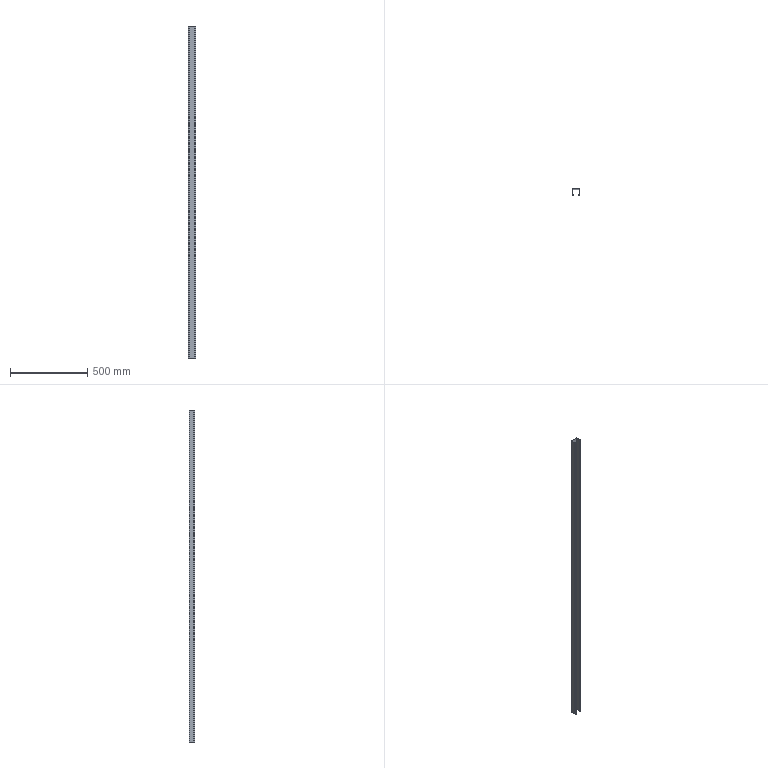Part | STEP file | 31E-01027QY25 | 1 solid | 28 faces | box 50 x 38.192 x 2150 mm | volume 353976 mm3 | plane 16 | cylinder 12 | commonest cylinder face diameters 1 x4 2 x4 4 x2 26 x2
STEP:
#1=CARTESIAN_POINT('',(27.993,8.298,1075.));
#2=VERTEX_POINT('',#1);
#3=CARTESIAN_POINT('',(32.281,3.187,1075.));
#4=VERTEX_POINT('',#3);
#5=CARTESIAN_POINT('',(30.137,5.743,1075.));
#6=DIRECTION('',(0.6428,-0.766,0.));
#7=VECTOR('',#6,1.);
#8=LINE('',#5,#7);
#9=EDGE_CURVE('',#2,#4,#8,.T.);
#10=ORIENTED_EDGE('',*,*,#9,.F.);
#11=CARTESIAN_POINT('',(27.993,8.298,-1075.));
#12=VERTEX_POINT('',#11);
#13=CARTESIAN_POINT('',(27.993,8.298,0.));
#14=DIRECTION('',(0.,0.,-1.));
#15=VECTOR('',#14,1.);
#16=LINE('',#13,#15);
#17=EDGE_CURVE('',#2,#12,#16,.T.);
#18=ORIENTED_EDGE('',*,*,#17,.T.);
#19=CARTESIAN_POINT('',(32.281,3.187,-1075.));
#20=VERTEX_POINT('',#19);
#21=CARTESIAN_POINT('',(30.137,5.743,-1075.));
#22=DIRECTION('',(0.6428,-0.766,0.));
#23=VECTOR('',#22,1.);
#24=LINE('',#21,#23);
#25=EDGE_CURVE('',#12,#20,#24,.T.);
#26=ORIENTED_EDGE('',*,*,#25,.T.);
#27=CARTESIAN_POINT('',(32.281,3.187,0.));
#28=DIRECTION('',(0.,0.,-1.));
#29=VECTOR('',#28,1.);
#30=LINE('',#27,#29);
#31=EDGE_CURVE('',#4,#20,#30,.T.);
#32=ORIENTED_EDGE('',*,*,#31,.F.);
#33=EDGE_LOOP('',(#10,#18,#26,#32));
#34=FACE_OUTER_BOUND('',#33,.T.);
#35=CARTESIAN_POINT('',(27.525,8.856,1075.));
#36=DIRECTION('',(0.766,0.6428,0.));
#37=DIRECTION('',(-0.6428,0.766,0.));
#38=AXIS2_PLACEMENT_3D('',#35,#36,#37);
#39=PLANE('',#38);
#40=ADVANCED_FACE('',(#34),#39,.F.);
#41=CARTESIAN_POINT('',(76.525,38.856,1075.));
#42=VERTEX_POINT('',#41);
#43=CARTESIAN_POINT('',(28.525,38.856,1075.));
#44=VERTEX_POINT('',#43);
#45=CARTESIAN_POINT('',(52.525,38.856,1075.));
#46=DIRECTION('',(-1.,0.,0.));
#47=VECTOR('',#46,1.);
#48=LINE('',#45,#47);
#49=EDGE_CURVE('',#42,#44,#48,.T.);
#50=ORIENTED_EDGE('',*,*,#49,.T.);
#51=CARTESIAN_POINT('',(27.525,37.856,1075.));
#52=VERTEX_POINT('',#51);
#53=CARTESIAN_POINT('',(28.525,37.856,1075.));
#54=DIRECTION('',(0.,0.,1.));
#55=AXIS2_PLACEMENT_3D('',#53,#54,$);
#56=CIRCLE('',#55,1.);
#57=EDGE_CURVE('',#44,#52,#56,.T.);
#58=ORIENTED_EDGE('',*,*,#57,.T.);
#59=CARTESIAN_POINT('',(27.525,9.584,1075.));
#60=VERTEX_POINT('',#59);
#61=CARTESIAN_POINT('',(27.525,23.72,1075.));
#62=DIRECTION('',(0.,-1.,0.));
#63=VECTOR('',#62,1.);
#64=LINE('',#61,#63);
#65=EDGE_CURVE('',#52,#60,#64,.T.);
#66=ORIENTED_EDGE('',*,*,#65,.T.);
#67=CARTESIAN_POINT('',(29.525,9.584,1075.));
#68=DIRECTION('',(0.,0.,1.));
#69=AXIS2_PLACEMENT_3D('',#67,#68,$);
#70=CIRCLE('',#69,2.);
#71=EDGE_CURVE('',#60,#2,#70,.T.);
#72=ORIENTED_EDGE('',*,*,#71,.T.);
#73=ORIENTED_EDGE('',*,*,#9,.T.);
#74=CARTESIAN_POINT('',(28.342,2.493,1075.));
#75=VERTEX_POINT('',#74);
#76=CARTESIAN_POINT('',(30.312,2.84,1075.));
#77=DIRECTION('',(-0.9848,-0.1736,0.));
#78=VECTOR('',#77,1.);
#79=LINE('',#76,#78);
#80=EDGE_CURVE('',#4,#75,#79,.T.);
#81=ORIENTED_EDGE('',*,*,#80,.T.);
#82=CARTESIAN_POINT('',(32.653,0.6877,1075.));
#83=VERTEX_POINT('',#82);
#84=CARTESIAN_POINT('',(35.437,13.386,1075.));
#85=DIRECTION('',(0.,0.,1.));
#86=AXIS2_PLACEMENT_3D('',#84,#85,$);
#87=CIRCLE('',#86,13.);
#88=EDGE_CURVE('',#75,#83,#87,.T.);
#89=ORIENTED_EDGE('',*,*,#88,.T.);
#90=CARTESIAN_POINT('',(33.867,1.665,1075.));
#91=VERTEX_POINT('',#90);
#92=CARTESIAN_POINT('',(32.867,1.665,1075.));
#93=DIRECTION('',(0.,0.,1.));
#94=AXIS2_PLACEMENT_3D('',#92,#93,$);
#95=CIRCLE('',#94,1.);
#96=EDGE_CURVE('',#83,#91,#95,.T.);
#97=ORIENTED_EDGE('',*,*,#96,.T.);
#98=CARTESIAN_POINT('',(33.867,2.983,1075.));
#99=VERTEX_POINT('',#98);
#100=CARTESIAN_POINT('',(33.867,2.324,1075.));
#101=DIRECTION('',(0.,1.,0.));
#102=VECTOR('',#101,1.);
#103=LINE('',#100,#102);
#104=EDGE_CURVE('',#91,#99,#103,.T.);
#105=ORIENTED_EDGE('',*,*,#104,.T.);
#106=CARTESIAN_POINT('',(33.75,3.304,1075.));
#107=VERTEX_POINT('',#106);
#108=CARTESIAN_POINT('',(33.367,2.983,1075.));
#109=DIRECTION('',(0.,0.,1.));
#110=AXIS2_PLACEMENT_3D('',#108,#109,$);
#111=CIRCLE('',#110,0.5);
#112=EDGE_CURVE('',#99,#107,#111,.T.);
#113=ORIENTED_EDGE('',*,*,#112,.T.);
#114=CARTESIAN_POINT('',(28.725,9.293,1075.));
#115=VERTEX_POINT('',#114);
#116=CARTESIAN_POINT('',(31.237,6.298,1075.));
#117=DIRECTION('',(-0.6428,0.766,0.));
#118=VECTOR('',#117,1.);
#119=LINE('',#116,#118);
#120=EDGE_CURVE('',#107,#115,#119,.T.);
#121=ORIENTED_EDGE('',*,*,#120,.T.);
#122=CARTESIAN_POINT('',(28.725,37.156,1075.));
#123=VERTEX_POINT('',#122);
#124=CARTESIAN_POINT('',(28.725,23.225,1075.));
#125=DIRECTION('',(0.,1.,0.));
#126=VECTOR('',#125,1.);
#127=LINE('',#124,#126);
#128=EDGE_CURVE('',#115,#123,#127,.T.);
#129=ORIENTED_EDGE('',*,*,#128,.T.);
#130=CARTESIAN_POINT('',(29.225,37.656,1075.));
#131=VERTEX_POINT('',#130);
#132=CARTESIAN_POINT('',(28.725,37.156,1075.));
#133=CARTESIAN_POINT('',(28.725,37.219,1075.));
#134=CARTESIAN_POINT('',(28.735,37.282,1075.));
#135=CARTESIAN_POINT('',(28.754,37.343,1075.));
#136=CARTESIAN_POINT('',(28.812,37.456,1075.));
#137=CARTESIAN_POINT('',(28.902,37.546,1075.));
#138=CARTESIAN_POINT('',(28.954,37.583,1075.));
#139=CARTESIAN_POINT('',(29.039,37.627,1075.));
#140=CARTESIAN_POINT('',(29.131,37.649,1075.));
#141=CARTESIAN_POINT('',(29.162,37.654,1075.));
#142=CARTESIAN_POINT('',(29.193,37.656,1075.));
#143=CARTESIAN_POINT('',(29.225,37.656,1075.));
#144=B_SPLINE_CURVE_WITH_KNOTS('',5,(#132,#133,#134,#135,#136,#137,#138,#139,#140,#141,#142,#143),.UNSPECIFIED.,.F.,.U.,(6,3,3,6),(0.,0.4443,0.8886,1.11),.UNSPECIFIED.);
#145=EDGE_CURVE('',#123,#131,#144,.T.);
#146=ORIENTED_EDGE('',*,*,#145,.T.);
#147=CARTESIAN_POINT('',(75.825,37.656,1075.));
#148=VERTEX_POINT('',#147);
#149=CARTESIAN_POINT('',(52.525,37.656,1075.));
#150=DIRECTION('',(1.,0.,0.));
#151=VECTOR('',#150,1.);
#152=LINE('',#149,#151);
#153=EDGE_CURVE('',#131,#148,#152,.T.);
#154=ORIENTED_EDGE('',*,*,#153,.T.);
#155=CARTESIAN_POINT('',(76.325,37.156,1075.));
#156=VERTEX_POINT('',#155);
#157=CARTESIAN_POINT('',(75.825,37.656,1075.));
#158=CARTESIAN_POINT('',(75.888,37.656,1075.));
#159=CARTESIAN_POINT('',(75.95,37.646,1075.));
#160=CARTESIAN_POINT('',(76.011,37.627,1075.));
#161=CARTESIAN_POINT('',(76.124,37.569,1075.));
#162=CARTESIAN_POINT('',(76.214,37.479,1075.));
#163=CARTESIAN_POINT('',(76.252,37.427,1075.));
#164=CARTESIAN_POINT('',(76.295,37.342,1075.));
#165=CARTESIAN_POINT('',(76.317,37.25,1075.));
#166=CARTESIAN_POINT('',(76.322,37.219,1075.));
#167=CARTESIAN_POINT('',(76.325,37.187,1075.));
#168=CARTESIAN_POINT('',(76.325,37.156,1075.));
#169=B_SPLINE_CURVE_WITH_KNOTS('',5,(#157,#158,#159,#160,#161,#162,#163,#164,#165,#166,#167,#168),.UNSPECIFIED.,.F.,.U.,(6,3,3,6),(0.,0.4443,0.8886,1.11),.UNSPECIFIED.);
#170=EDGE_CURVE('',#148,#156,#169,.T.);
#171=ORIENTED_EDGE('',*,*,#170,.T.);
#172=CARTESIAN_POINT('',(76.325,9.293,1075.));
#173=VERTEX_POINT('',#172);
#174=CARTESIAN_POINT('',(76.325,23.225,1075.));
#175=DIRECTION('',(0.,-1.,0.));
#176=VECTOR('',#175,1.);
#177=LINE('',#174,#176);
#178=EDGE_CURVE('',#156,#173,#177,.T.);
#179=ORIENTED_EDGE('',*,*,#178,.T.);
#180=CARTESIAN_POINT('',(71.299,3.304,1075.));
#181=VERTEX_POINT('',#180);
#182=CARTESIAN_POINT('',(73.812,6.298,1075.));
#183=DIRECTION('',(-0.6428,-0.766,0.));
#184=VECTOR('',#183,1.);
#185=LINE('',#182,#184);
#186=EDGE_CURVE('',#173,#181,#185,.T.);
#187=ORIENTED_EDGE('',*,*,#186,.T.);
#188=CARTESIAN_POINT('',(71.182,2.983,1075.));
#189=VERTEX_POINT('',#188);
#190=CARTESIAN_POINT('',(71.682,2.983,1075.));
#191=DIRECTION('',(0.,0.,1.));
#192=AXIS2_PLACEMENT_3D('',#190,#191,$);
#193=CIRCLE('',#192,0.5);
#194=EDGE_CURVE('',#181,#189,#193,.T.);
#195=ORIENTED_EDGE('',*,*,#194,.T.);
#196=CARTESIAN_POINT('',(71.182,1.665,1075.));
#197=VERTEX_POINT('',#196);
#198=CARTESIAN_POINT('',(71.182,2.324,1075.));
#199=DIRECTION('',(0.,-1.,0.));
#200=VECTOR('',#199,1.);
#201=LINE('',#198,#200);
#202=EDGE_CURVE('',#189,#197,#201,.T.);
#203=ORIENTED_EDGE('',*,*,#202,.T.);
#204=CARTESIAN_POINT('',(72.397,0.6877,1075.));
#205=VERTEX_POINT('',#204);
#206=CARTESIAN_POINT('',(72.182,1.665,1075.));
#207=DIRECTION('',(0.,0.,1.));
#208=AXIS2_PLACEMENT_3D('',#206,#207,$);
#209=CIRCLE('',#208,1.);
#210=EDGE_CURVE('',#197,#205,#209,.T.);
#211=ORIENTED_EDGE('',*,*,#210,.T.);
#212=CARTESIAN_POINT('',(76.707,2.493,1075.));
#213=VERTEX_POINT('',#212);
#214=CARTESIAN_POINT('',(69.613,13.386,1075.));
#215=DIRECTION('',(0.,0.,1.));
#216=AXIS2_PLACEMENT_3D('',#214,#215,$);
#217=CIRCLE('',#216,13.);
#218=EDGE_CURVE('',#205,#213,#217,.T.);
#219=ORIENTED_EDGE('',*,*,#218,.T.);
#220=CARTESIAN_POINT('',(72.768,3.187,1075.));
#221=VERTEX_POINT('',#220);
#222=CARTESIAN_POINT('',(74.738,2.84,1075.));
#223=DIRECTION('',(-0.9848,0.1736,0.));
#224=VECTOR('',#223,1.);
#225=LINE('',#222,#224);
#226=EDGE_CURVE('',#213,#221,#225,.T.);
#227=ORIENTED_EDGE('',*,*,#226,.T.);
#228=CARTESIAN_POINT('',(77.057,8.298,1075.));
#229=VERTEX_POINT('',#228);
#230=CARTESIAN_POINT('',(74.912,5.743,1075.));
#231=DIRECTION('',(0.6428,0.766,0.));
#232=VECTOR('',#231,1.);
#233=LINE('',#230,#232);
#234=EDGE_CURVE('',#221,#229,#233,.T.);
#235=ORIENTED_EDGE('',*,*,#234,.T.);
#236=CARTESIAN_POINT('',(77.525,9.584,1075.));
#237=VERTEX_POINT('',#236);
#238=CARTESIAN_POINT('',(75.525,9.584,1075.));
#239=DIRECTION('',(0.,0.,1.));
#240=AXIS2_PLACEMENT_3D('',#238,#239,$);
#241=CIRCLE('',#240,2.);
#242=EDGE_CURVE('',#229,#237,#241,.T.);
#243=ORIENTED_EDGE('',*,*,#242,.T.);
#244=CARTESIAN_POINT('',(77.525,37.856,1075.));
#245=VERTEX_POINT('',#244);
#246=CARTESIAN_POINT('',(77.525,23.72,1075.));
#247=DIRECTION('',(0.,1.,0.));
#248=VECTOR('',#247,1.);
#249=LINE('',#246,#248);
#250=EDGE_CURVE('',#237,#245,#249,.T.);
#251=ORIENTED_EDGE('',*,*,#250,.T.);
#252=CARTESIAN_POINT('',(76.525,37.856,1075.));
#253=DIRECTION('',(0.,0.,1.));
#254=AXIS2_PLACEMENT_3D('',#252,#253,$);
#255=CIRCLE('',#254,1.);
#256=EDGE_CURVE('',#245,#42,#255,.T.);
#257=ORIENTED_EDGE('',*,*,#256,.T.);
#258=EDGE_LOOP('',(#50,#58,#66,#72,#73,#81,#89,#97,#105,#113,#121,#129,#146,#154,#171,#179,#187,#195,#203,#211,#219,#227,#235,#243,#251,#257));
#259=FACE_OUTER_BOUND('',#258,.T.);
#260=CARTESIAN_POINT('',(35.437,13.386,1075.));
#261=DIRECTION('',(0.,0.,1.));
#262=DIRECTION('',(1.,0.,0.));
#263=AXIS2_PLACEMENT_3D('',#260,#261,#262);
#264=PLANE('',#263);
#265=ADVANCED_FACE('',(#259),#264,.T.);
#266=ORIENTED_EDGE('',*,*,#71,.F.);
#267=CARTESIAN_POINT('',(27.525,9.584,-1075.));
#268=VERTEX_POINT('',#267);
#269=CARTESIAN_POINT('',(27.525,9.584,1075.));
#270=DIRECTION('',(0.,0.,-1.));
#271=VECTOR('',#270,1.);
#272=LINE('',#269,#271);
#273=EDGE_CURVE('',#268,#60,#272,.F.);
#274=ORIENTED_EDGE('',*,*,#273,.F.);
#275=CARTESIAN_POINT('',(29.525,9.584,-1075.));
#276=DIRECTION('',(0.,0.,-1.));
#277=AXIS2_PLACEMENT_3D('',#275,#276,$);
#278=CIRCLE('',#277,2.);
#279=EDGE_CURVE('',#12,#268,#278,.T.);
#280=ORIENTED_EDGE('',*,*,#279,.F.);
#281=ORIENTED_EDGE('',*,*,#17,.F.);
#282=EDGE_LOOP('',(#266,#274,#280,#281));
#283=FACE_OUTER_BOUND('',#282,.T.);
#284=CARTESIAN_POINT('',(29.525,9.584,1075.));
#285=DIRECTION('',(0.,0.,-1.));
#286=DIRECTION('',(1.,0.,0.));
#287=AXIS2_PLACEMENT_3D('',#284,#285,#286);
#288=CYLINDRICAL_SURFACE('',#287,2.);
#289=ADVANCED_FACE('',(#283),#288,.T.);
#290=CARTESIAN_POINT('',(27.525,37.856,-1075.));
#291=VERTEX_POINT('',#290);
#292=CARTESIAN_POINT('',(28.525,38.856,-1075.));
#293=VERTEX_POINT('',#292);
#294=CARTESIAN_POINT('',(27.525,37.856,-1075.));
#295=CARTESIAN_POINT('',(27.525,37.954,-1075.));
#296=CARTESIAN_POINT('',(27.537,38.052,-1075.));
#297=CARTESIAN_POINT('',(27.561,38.148,-1075.));
#298=CARTESIAN_POINT('',(27.632,38.332,-1075.));
#299=CARTESIAN_POINT('',(27.745,38.494,-1075.));
#300=CARTESIAN_POINT('',(27.812,38.567,-1075.));
#301=CARTESIAN_POINT('',(27.961,38.696,-1075.));
#302=CARTESIAN_POINT('',(28.137,38.786,-1075.));
#303=CARTESIAN_POINT('',(28.23,38.819,-1075.));
#304=CARTESIAN_POINT('',(28.346,38.846,-1075.));
#305=CARTESIAN_POINT('',(28.464,38.855,-1075.));
#306=CARTESIAN_POINT('',(28.484,38.856,-1075.));
#307=CARTESIAN_POINT('',(28.505,38.856,-1075.));
#308=CARTESIAN_POINT('',(28.525,38.856,-1075.));
#309=B_SPLINE_CURVE_WITH_KNOTS('',5,(#294,#295,#296,#297,#298,#299,#300,#301,#302,#303,#304,#305,#306,#307,#308),.UNSPECIFIED.,.F.,.U.,(6,3,3,3,6),(0.,0.6928,1.386,2.078,2.221),.UNSPECIFIED.);
#310=EDGE_CURVE('',#291,#293,#309,.T.);
#311=ORIENTED_EDGE('',*,*,#310,.T.);
#312=CARTESIAN_POINT('',(76.525,38.856,-1075.));
#313=VERTEX_POINT('',#312);
#314=CARTESIAN_POINT('',(52.525,38.856,-1075.));
#315=DIRECTION('',(-1.,0.,0.));
#316=VECTOR('',#315,1.);
#317=LINE('',#314,#316);
#318=EDGE_CURVE('',#313,#293,#317,.T.);
#319=ORIENTED_EDGE('',*,*,#318,.F.);
#320=CARTESIAN_POINT('',(77.525,37.856,-1075.));
#321=VERTEX_POINT('',#320);
#322=CARTESIAN_POINT('',(76.525,38.856,-1075.));
#323=CARTESIAN_POINT('',(76.623,38.856,-1075.));
#324=CARTESIAN_POINT('',(76.721,38.844,-1075.));
#325=CARTESIAN_POINT('',(76.817,38.82,-1075.));
#326=CARTESIAN_POINT('',(77.001,38.749,-1075.));
#327=CARTESIAN_POINT('',(77.163,38.636,-1075.));
#328=CARTESIAN_POINT('',(77.236,38.569,-1075.));
#329=CARTESIAN_POINT('',(77.365,38.42,-1075.));
#330=CARTESIAN_POINT('',(77.454,38.244,-1075.));
#331=CARTESIAN_POINT('',(77.488,38.151,-1075.));
#332=CARTESIAN_POINT('',(77.514,38.035,-1075.));
#333=CARTESIAN_POINT('',(77.523,37.917,-1075.));
#334=CARTESIAN_POINT('',(77.524,37.897,-1075.));
#335=CARTESIAN_POINT('',(77.525,37.876,-1075.));
#336=CARTESIAN_POINT('',(77.525,37.856,-1075.));
#337=B_SPLINE_CURVE_WITH_KNOTS('',5,(#322,#323,#324,#325,#326,#327,#328,#329,#330,#331,#332,#333,#334,#335,#336),.UNSPECIFIED.,.F.,.U.,(6,3,3,3,6),(0.,0.6928,1.386,2.078,2.221),.UNSPECIFIED.);
#338=EDGE_CURVE('',#313,#321,#337,.T.);
#339=ORIENTED_EDGE('',*,*,#338,.T.);
#340=CARTESIAN_POINT('',(77.525,9.584,-1075.));
#341=VERTEX_POINT('',#340);
#342=CARTESIAN_POINT('',(77.525,23.72,-1075.));
#343=DIRECTION('',(0.,1.,0.));
#344=VECTOR('',#343,1.);
#345=LINE('',#342,#344);
#346=EDGE_CURVE('',#341,#321,#345,.T.);
#347=ORIENTED_EDGE('',*,*,#346,.F.);
#348=CARTESIAN_POINT('',(77.057,8.298,-1075.));
#349=VERTEX_POINT('',#348);
#350=CARTESIAN_POINT('',(77.525,9.584,-1075.));
#351=CARTESIAN_POINT('',(77.525,9.361,-1075.));
#352=CARTESIAN_POINT('',(77.494,9.137,-1075.));
#353=CARTESIAN_POINT('',(77.431,8.92,-1075.));
#354=CARTESIAN_POINT('',(77.316,8.662,-1075.));
#355=CARTESIAN_POINT('',(77.16,8.431,-1075.));
#356=CARTESIAN_POINT('',(77.127,8.385,-1075.));
#357=CARTESIAN_POINT('',(77.093,8.341,-1075.));
#358=CARTESIAN_POINT('',(77.057,8.298,-1075.));
#359=B_SPLINE_CURVE_WITH_KNOTS('',5,(#350,#351,#352,#353,#354,#355,#356,#357,#358),.UNSPECIFIED.,.F.,.U.,(6,3,6),(0.,1.58,1.974),.UNSPECIFIED.);
#360=EDGE_CURVE('',#341,#349,#359,.T.);
#361=ORIENTED_EDGE('',*,*,#360,.T.);
#362=CARTESIAN_POINT('',(72.768,3.187,-1075.));
#363=VERTEX_POINT('',#362);
#364=CARTESIAN_POINT('',(74.912,5.743,-1075.));
#365=DIRECTION('',(0.6428,0.766,0.));
#366=VECTOR('',#365,1.);
#367=LINE('',#364,#366);
#368=EDGE_CURVE('',#363,#349,#367,.T.);
#369=ORIENTED_EDGE('',*,*,#368,.F.);
#370=CARTESIAN_POINT('',(76.707,2.493,-1075.));
#371=VERTEX_POINT('',#370);
#372=CARTESIAN_POINT('',(74.738,2.84,-1075.));
#373=DIRECTION('',(-0.9848,0.1736,0.));
#374=VECTOR('',#373,1.);
#375=LINE('',#372,#374);
#376=EDGE_CURVE('',#371,#363,#375,.T.);
#377=ORIENTED_EDGE('',*,*,#376,.F.);
#378=CARTESIAN_POINT('',(72.397,0.6877,-1075.));
#379=VERTEX_POINT('',#378);
#380=CARTESIAN_POINT('',(69.613,13.386,-1075.));
#381=DIRECTION('',(0.,0.,1.));
#382=AXIS2_PLACEMENT_3D('',#380,#381,$);
#383=CIRCLE('',#382,13.);
#384=EDGE_CURVE('',#379,#371,#383,.T.);
#385=ORIENTED_EDGE('',*,*,#384,.F.);
#386=CARTESIAN_POINT('',(71.182,1.665,-1075.));
#387=VERTEX_POINT('',#386);
#388=CARTESIAN_POINT('',(72.182,1.665,-1075.));
#389=DIRECTION('',(0.,0.,1.));
#390=AXIS2_PLACEMENT_3D('',#388,#389,$);
#391=CIRCLE('',#390,1.);
#392=EDGE_CURVE('',#387,#379,#391,.T.);
#393=ORIENTED_EDGE('',*,*,#392,.F.);
#394=CARTESIAN_POINT('',(71.182,2.983,-1075.));
#395=VERTEX_POINT('',#394);
#396=CARTESIAN_POINT('',(71.182,2.324,-1075.));
#397=DIRECTION('',(0.,-1.,0.));
#398=VECTOR('',#397,1.);
#399=LINE('',#396,#398);
#400=EDGE_CURVE('',#395,#387,#399,.T.);
#401=ORIENTED_EDGE('',*,*,#400,.F.);
#402=CARTESIAN_POINT('',(71.299,3.304,-1075.));
#403=VERTEX_POINT('',#402);
#404=CARTESIAN_POINT('',(71.182,2.983,-1075.));
#405=CARTESIAN_POINT('',(71.182,3.038,-1075.));
#406=CARTESIAN_POINT('',(71.19,3.094,-1075.));
#407=CARTESIAN_POINT('',(71.206,3.149,-1075.));
#408=CARTESIAN_POINT('',(71.235,3.213,-1075.));
#409=CARTESIAN_POINT('',(71.274,3.271,-1075.));
#410=CARTESIAN_POINT('',(71.282,3.282,-1075.));
#411=CARTESIAN_POINT('',(71.29,3.293,-1075.));
#412=CARTESIAN_POINT('',(71.299,3.304,-1075.));
#413=B_SPLINE_CURVE_WITH_KNOTS('',5,(#404,#405,#406,#407,#408,#409,#410,#411,#412),.UNSPECIFIED.,.F.,.U.,(6,3,6),(0.,0.3949,0.4936),.UNSPECIFIED.);
#414=EDGE_CURVE('',#395,#403,#413,.T.);
#415=ORIENTED_EDGE('',*,*,#414,.T.);
#416=CARTESIAN_POINT('',(76.325,9.293,-1075.));
#417=VERTEX_POINT('',#416);
#418=CARTESIAN_POINT('',(73.812,6.298,-1075.));
#419=DIRECTION('',(-0.6428,-0.766,0.));
#420=VECTOR('',#419,1.);
#421=LINE('',#418,#420);
#422=EDGE_CURVE('',#417,#403,#421,.T.);
#423=ORIENTED_EDGE('',*,*,#422,.F.);
#424=CARTESIAN_POINT('',(76.325,37.156,-1075.));
#425=VERTEX_POINT('',#424);
#426=CARTESIAN_POINT('',(76.325,23.225,-1075.));
#427=DIRECTION('',(0.,-1.,0.));
#428=VECTOR('',#427,1.);
#429=LINE('',#426,#428);
#430=EDGE_CURVE('',#425,#417,#429,.T.);
#431=ORIENTED_EDGE('',*,*,#430,.F.);
#432=CARTESIAN_POINT('',(75.825,37.656,-1075.));
#433=VERTEX_POINT('',#432);
#434=CARTESIAN_POINT('',(75.825,37.156,-1075.));
#435=DIRECTION('',(0.,0.,1.));
#436=AXIS2_PLACEMENT_3D('',#434,#435,$);
#437=CIRCLE('',#436,0.5);
#438=EDGE_CURVE('',#425,#433,#437,.T.);
#439=ORIENTED_EDGE('',*,*,#438,.T.);
#440=CARTESIAN_POINT('',(29.225,37.656,-1075.));
#441=VERTEX_POINT('',#440);
#442=CARTESIAN_POINT('',(52.525,37.656,-1075.));
#443=DIRECTION('',(1.,0.,0.));
#444=VECTOR('',#443,1.);
#445=LINE('',#442,#444);
#446=EDGE_CURVE('',#441,#433,#445,.T.);
#447=ORIENTED_EDGE('',*,*,#446,.F.);
#448=CARTESIAN_POINT('',(28.725,37.156,-1075.));
#449=VERTEX_POINT('',#448);
#450=CARTESIAN_POINT('',(29.225,37.156,-1075.));
#451=DIRECTION('',(0.,0.,1.));
#452=AXIS2_PLACEMENT_3D('',#450,#451,$);
#453=CIRCLE('',#452,0.5);
#454=EDGE_CURVE('',#441,#449,#453,.T.);
#455=ORIENTED_EDGE('',*,*,#454,.T.);
#456=CARTESIAN_POINT('',(28.725,9.293,-1075.));
#457=VERTEX_POINT('',#456);
#458=CARTESIAN_POINT('',(28.725,23.225,-1075.));
#459=DIRECTION('',(0.,1.,0.));
#460=VECTOR('',#459,1.);
#461=LINE('',#458,#460);
#462=EDGE_CURVE('',#457,#449,#461,.T.);
#463=ORIENTED_EDGE('',*,*,#462,.F.);
#464=CARTESIAN_POINT('',(33.75,3.304,-1075.));
#465=VERTEX_POINT('',#464);
#466=CARTESIAN_POINT('',(31.237,6.298,-1075.));
#467=DIRECTION('',(-0.6428,0.766,0.));
#468=VECTOR('',#467,1.);
#469=LINE('',#466,#468);
#470=EDGE_CURVE('',#465,#457,#469,.T.);
#471=ORIENTED_EDGE('',*,*,#470,.F.);
#472=CARTESIAN_POINT('',(33.867,2.983,-1075.));
#473=VERTEX_POINT('',#472);
#474=CARTESIAN_POINT('',(33.75,3.304,-1075.));
#475=CARTESIAN_POINT('',(33.786,3.261,-1075.));
#476=CARTESIAN_POINT('',(33.816,3.213,-1075.));
#477=CARTESIAN_POINT('',(33.839,3.162,-1075.));
#478=CARTESIAN_POINT('',(33.858,3.094,-1075.));
#479=CARTESIAN_POINT('',(33.866,3.024,-1075.));
#480=CARTESIAN_POINT('',(33.867,3.01,-1075.));
#481=CARTESIAN_POINT('',(33.867,2.997,-1075.));
#482=CARTESIAN_POINT('',(33.867,2.983,-1075.));
#483=B_SPLINE_CURVE_WITH_KNOTS('',5,(#474,#475,#476,#477,#478,#479,#480,#481,#482),.UNSPECIFIED.,.F.,.U.,(6,3,6),(0.,0.3949,0.4936),.UNSPECIFIED.);
#484=EDGE_CURVE('',#465,#473,#483,.T.);
#485=ORIENTED_EDGE('',*,*,#484,.T.);
#486=CARTESIAN_POINT('',(33.867,1.665,-1075.));
#487=VERTEX_POINT('',#486);
#488=CARTESIAN_POINT('',(33.867,2.324,-1075.));
#489=DIRECTION('',(0.,1.,0.));
#490=VECTOR('',#489,1.);
#491=LINE('',#488,#490);
#492=EDGE_CURVE('',#487,#473,#491,.T.);
#493=ORIENTED_EDGE('',*,*,#492,.F.);
#494=CARTESIAN_POINT('',(32.653,0.6877,-1075.));
#495=VERTEX_POINT('',#494);
#496=CARTESIAN_POINT('',(32.867,1.665,-1075.));
#497=DIRECTION('',(0.,0.,1.));
#498=AXIS2_PLACEMENT_3D('',#496,#497,$);
#499=CIRCLE('',#498,1.);
#500=EDGE_CURVE('',#495,#487,#499,.T.);
#501=ORIENTED_EDGE('',*,*,#500,.F.);
#502=CARTESIAN_POINT('',(28.342,2.493,-1075.));
#503=VERTEX_POINT('',#502);
#504=CARTESIAN_POINT('',(35.437,13.386,-1075.));
#505=DIRECTION('',(0.,0.,1.));
#506=AXIS2_PLACEMENT_3D('',#504,#505,$);
#507=CIRCLE('',#506,13.);
#508=EDGE_CURVE('',#503,#495,#507,.T.);
#509=ORIENTED_EDGE('',*,*,#508,.F.);
#510=CARTESIAN_POINT('',(30.312,2.84,-1075.));
#511=DIRECTION('',(-0.9848,-0.1736,0.));
#512=VECTOR('',#511,1.);
#513=LINE('',#510,#512);
#514=EDGE_CURVE('',#20,#503,#513,.T.);
#515=ORIENTED_EDGE('',*,*,#514,.F.);
#516=ORIENTED_EDGE('',*,*,#25,.F.);
#517=ORIENTED_EDGE('',*,*,#279,.T.);
#518=CARTESIAN_POINT('',(27.525,23.72,-1075.));
#519=DIRECTION('',(0.,-1.,0.));
#520=VECTOR('',#519,1.);
#521=LINE('',#518,#520);
#522=EDGE_CURVE('',#291,#268,#521,.T.);
#523=ORIENTED_EDGE('',*,*,#522,.F.);
#524=EDGE_LOOP('',(#311,#319,#339,#347,#361,#369,#377,#385,#393,#401,#415,#423,#431,#439,#447,#455,#463,#471,#485,#493,#501,#509,#515,#516,#517,#523));
#525=FACE_OUTER_BOUND('',#524,.T.);
#526=CARTESIAN_POINT('',(35.437,13.386,-1075.));
#527=DIRECTION('',(0.,0.,1.));
#528=DIRECTION('',(1.,0.,0.));
#529=AXIS2_PLACEMENT_3D('',#526,#527,#528);
#530=PLANE('',#529);
#531=ADVANCED_FACE('',(#525),#530,.F.);
#532=ORIENTED_EDGE('',*,*,#514,.T.);
#533=CARTESIAN_POINT('',(28.342,2.493,0.));
#534=DIRECTION('',(0.,0.,-1.));
#535=VECTOR('',#534,1.);
#536=LINE('',#533,#535);
#537=EDGE_CURVE('',#75,#503,#536,.T.);
#538=ORIENTED_EDGE('',*,*,#537,.F.);
#539=ORIENTED_EDGE('',*,*,#80,.F.);
#540=ORIENTED_EDGE('',*,*,#31,.T.);
#541=EDGE_LOOP('',(#532,#538,#539,#540));
#542=FACE_OUTER_BOUND('',#541,.T.);
#543=CARTESIAN_POINT('',(32.281,3.187,1075.));
#544=DIRECTION('',(0.1736,-0.9848,0.));
#545=DIRECTION('',(0.9848,0.1736,0.));
#546=AXIS2_PLACEMENT_3D('',#543,#544,#545);
#547=PLANE('',#546);
#548=ADVANCED_FACE('',(#542),#547,.F.);
#549=ORIENTED_EDGE('',*,*,#318,.T.);
#550=CARTESIAN_POINT('',(28.525,38.856,0.));
#551=DIRECTION('',(0.,0.,1.));
#552=VECTOR('',#551,1.);
#553=LINE('',#550,#552);
#554=EDGE_CURVE('',#293,#44,#553,.T.);
#555=ORIENTED_EDGE('',*,*,#554,.T.);
#556=ORIENTED_EDGE('',*,*,#49,.F.);
#557=CARTESIAN_POINT('',(76.525,38.856,0.));
#558=DIRECTION('',(0.,0.,-1.));
#559=VECTOR('',#558,1.);
#560=LINE('',#557,#559);
#561=EDGE_CURVE('',#42,#313,#560,.T.);
#562=ORIENTED_EDGE('',*,*,#561,.T.);
#563=EDGE_LOOP('',(#549,#555,#556,#562));
#564=FACE_OUTER_BOUND('',#563,.T.);
#565=CARTESIAN_POINT('',(27.525,38.856,1075.));
#566=DIRECTION('',(0.,-1.,0.));
#567=DIRECTION('',(1.,0.,0.));
#568=AXIS2_PLACEMENT_3D('',#565,#566,#567);
#569=PLANE('',#568);
#570=ADVANCED_FACE('',(#564),#569,.F.);
#571=ORIENTED_EDGE('',*,*,#57,.F.);
#572=ORIENTED_EDGE('',*,*,#554,.F.);
#573=ORIENTED_EDGE('',*,*,#310,.F.);
#574=CARTESIAN_POINT('',(27.525,37.856,1075.));
#575=DIRECTION('',(0.,0.,-1.));
#576=VECTOR('',#575,1.);
#577=LINE('',#574,#576);
#578=EDGE_CURVE('',#52,#291,#577,.T.);
#579=ORIENTED_EDGE('',*,*,#578,.F.);
#580=EDGE_LOOP('',(#571,#572,#573,#579));
#581=FACE_OUTER_BOUND('',#580,.T.);
#582=CARTESIAN_POINT('',(28.525,37.856,1075.));
#583=DIRECTION('',(0.,0.,-1.));
#584=DIRECTION('',(-1.,0.,0.));
#585=AXIS2_PLACEMENT_3D('',#582,#583,#584);
#586=CYLINDRICAL_SURFACE('',#585,1.);
#587=ADVANCED_FACE('',(#581),#586,.T.);
#588=ORIENTED_EDGE('',*,*,#65,.F.);
#589=ORIENTED_EDGE('',*,*,#578,.T.);
#590=ORIENTED_EDGE('',*,*,#522,.T.);
#591=ORIENTED_EDGE('',*,*,#273,.T.);
#592=EDGE_LOOP('',(#588,#589,#590,#591));
#593=FACE_OUTER_BOUND('',#592,.T.);
#594=CARTESIAN_POINT('',(27.525,8.856,1075.));
#595=DIRECTION('',(1.,0.,0.));
#596=DIRECTION('',(0.,0.,-1.));
#597=AXIS2_PLACEMENT_3D('',#594,#595,#596);
#598=PLANE('',#597);
#599=ADVANCED_FACE('',(#593),#598,.F.);
#600=ORIENTED_EDGE('',*,*,#508,.T.);
#601=CARTESIAN_POINT('',(32.653,0.6877,1075.));
#602=DIRECTION('',(0.,0.,-1.));
#603=VECTOR('',#602,1.);
#604=LINE('',#601,#603);
#605=EDGE_CURVE('',#83,#495,#604,.T.);
#606=ORIENTED_EDGE('',*,*,#605,.F.);
#607=ORIENTED_EDGE('',*,*,#88,.F.);
#608=ORIENTED_EDGE('',*,*,#537,.T.);
#609=EDGE_LOOP('',(#600,#606,#607,#608));
#610=FACE_OUTER_BOUND('',#609,.T.);
#611=CARTESIAN_POINT('',(35.437,13.386,1075.));
#612=DIRECTION('',(0.,0.,-1.));
#613=DIRECTION('',(1.,0.,0.));
#614=AXIS2_PLACEMENT_3D('',#611,#612,#613);
#615=CYLINDRICAL_SURFACE('',#614,13.);
#616=ADVANCED_FACE('',(#610),#615,.T.);
#617=ORIENTED_EDGE('',*,*,#500,.T.);
#618=CARTESIAN_POINT('',(33.867,1.665,1075.));
#619=DIRECTION('',(0.,0.,-1.));
#620=VECTOR('',#619,1.);
#621=LINE('',#618,#620);
#622=EDGE_CURVE('',#91,#487,#621,.T.);
#623=ORIENTED_EDGE('',*,*,#622,.F.);
#624=ORIENTED_EDGE('',*,*,#96,.F.);
#625=ORIENTED_EDGE('',*,*,#605,.T.);
#626=EDGE_LOOP('',(#617,#623,#624,#625));
#627=FACE_OUTER_BOUND('',#626,.T.);
#628=CARTESIAN_POINT('',(32.867,1.665,1075.));
#629=DIRECTION('',(0.,0.,-1.));
#630=DIRECTION('',(1.,0.,0.));
#631=AXIS2_PLACEMENT_3D('',#628,#629,#630);
#632=CYLINDRICAL_SURFACE('',#631,1.);
#633=ADVANCED_FACE('',(#627),#632,.T.);
#634=ORIENTED_EDGE('',*,*,#492,.T.);
#635=CARTESIAN_POINT('',(33.867,2.983,0.));
#636=DIRECTION('',(0.,0.,1.));
#637=VECTOR('',#636,1.);
#638=LINE('',#635,#637);
#639=EDGE_CURVE('',#473,#99,#638,.T.);
#640=ORIENTED_EDGE('',*,*,#639,.T.);
#641=ORIENTED_EDGE('',*,*,#104,.F.);
#642=ORIENTED_EDGE('',*,*,#622,.T.);
#643=EDGE_LOOP('',(#634,#640,#641,#642));
#644=FACE_OUTER_BOUND('',#643,.T.);
#645=CARTESIAN_POINT('',(33.867,1.665,1075.));
#646=DIRECTION('',(-1.,0.,0.));
#647=DIRECTION('',(0.,0.,1.));
#648=AXIS2_PLACEMENT_3D('',#645,#646,#647);
#649=PLANE('',#648);
#650=ADVANCED_FACE('',(#644),#649,.F.);
#651=ORIENTED_EDGE('',*,*,#112,.F.);
#652=ORIENTED_EDGE('',*,*,#639,.F.);
#653=ORIENTED_EDGE('',*,*,#484,.F.);
#654=CARTESIAN_POINT('',(33.75,3.304,1075.));
#655=DIRECTION('',(0.,0.,-1.));
#656=VECTOR('',#655,1.);
#657=LINE('',#654,#656);
#658=EDGE_CURVE('',#107,#465,#657,.T.);
#659=ORIENTED_EDGE('',*,*,#658,.F.);
#660=EDGE_LOOP('',(#651,#652,#653,#659));
#661=FACE_OUTER_BOUND('',#660,.T.);
#662=CARTESIAN_POINT('',(33.367,2.983,1075.));
#663=DIRECTION('',(0.,0.,-1.));
#664=DIRECTION('',(-1.,0.,0.));
#665=AXIS2_PLACEMENT_3D('',#662,#663,#664);
#666=CYLINDRICAL_SURFACE('',#665,0.5);
#667=ADVANCED_FACE('',(#661),#666,.T.);
#668=ORIENTED_EDGE('',*,*,#120,.F.);
#669=ORIENTED_EDGE('',*,*,#658,.T.);
#670=ORIENTED_EDGE('',*,*,#470,.T.);
#671=CARTESIAN_POINT('',(28.725,9.293,0.));
#672=DIRECTION('',(0.,0.,-1.));
#673=VECTOR('',#672,1.);
#674=LINE('',#671,#673);
#675=EDGE_CURVE('',#115,#457,#674,.T.);
#676=ORIENTED_EDGE('',*,*,#675,.F.);
#677=EDGE_LOOP('',(#668,#669,#670,#676));
#678=FACE_OUTER_BOUND('',#677,.T.);
#679=CARTESIAN_POINT('',(28.725,9.293,1075.));
#680=DIRECTION('',(-0.766,-0.6428,0.));
#681=DIRECTION('',(0.6428,-0.766,0.));
#682=AXIS2_PLACEMENT_3D('',#679,#680,#681);
#683=PLANE('',#682);
#684=ADVANCED_FACE('',(#678),#683,.F.);
#685=ORIENTED_EDGE('',*,*,#462,.T.);
#686=CARTESIAN_POINT('',(28.725,37.156,0.));
#687=DIRECTION('',(0.,0.,1.));
#688=VECTOR('',#687,1.);
#689=LINE('',#686,#688);
#690=EDGE_CURVE('',#449,#123,#689,.T.);
#691=ORIENTED_EDGE('',*,*,#690,.T.);
#692=ORIENTED_EDGE('',*,*,#128,.F.);
#693=ORIENTED_EDGE('',*,*,#675,.T.);
#694=EDGE_LOOP('',(#685,#691,#692,#693));
#695=FACE_OUTER_BOUND('',#694,.T.);
#696=CARTESIAN_POINT('',(28.725,9.293,1075.));
#697=DIRECTION('',(-1.,0.,0.));
#698=DIRECTION('',(0.,0.,1.));
#699=AXIS2_PLACEMENT_3D('',#696,#697,#698);
#700=PLANE('',#699);
#701=ADVANCED_FACE('',(#695),#700,.F.);
#702=ORIENTED_EDGE('',*,*,#145,.F.);
#703=ORIENTED_EDGE('',*,*,#690,.F.);
#704=ORIENTED_EDGE('',*,*,#454,.F.);
#705=CARTESIAN_POINT('',(29.225,37.656,1075.));
#706=DIRECTION('',(0.,0.,1.));
#707=VECTOR('',#706,1.);
#708=LINE('',#705,#707);
#709=EDGE_CURVE('',#131,#441,#708,.F.);
#710=ORIENTED_EDGE('',*,*,#709,.F.);
#711=EDGE_LOOP('',(#702,#703,#704,#710));
#712=FACE_OUTER_BOUND('',#711,.T.);
#713=CARTESIAN_POINT('',(29.225,37.156,1075.));
#714=DIRECTION('',(0.,0.,1.));
#715=DIRECTION('',(1.,0.,0.));
#716=AXIS2_PLACEMENT_3D('',#713,#714,#715);
#717=CYLINDRICAL_SURFACE('',#716,0.5);
#718=ADVANCED_FACE('',(#712),#717,.F.);
#719=ORIENTED_EDGE('',*,*,#446,.T.);
#720=CARTESIAN_POINT('',(75.825,37.656,0.));
#721=DIRECTION('',(0.,0.,1.));
#722=VECTOR('',#721,1.);
#723=LINE('',#720,#722);
#724=EDGE_CURVE('',#433,#148,#723,.T.);
#725=ORIENTED_EDGE('',*,*,#724,.T.);
#726=ORIENTED_EDGE('',*,*,#153,.F.);
#727=ORIENTED_EDGE('',*,*,#709,.T.);
#728=EDGE_LOOP('',(#719,#725,#726,#727));
#729=FACE_OUTER_BOUND('',#728,.T.);
#730=CARTESIAN_POINT('',(28.725,37.656,1075.));
#731=DIRECTION('',(0.,1.,0.));
#732=DIRECTION('',(-1.,0.,0.));
#733=AXIS2_PLACEMENT_3D('',#730,#731,#732);
#734=PLANE('',#733);
#735=ADVANCED_FACE('',(#729),#734,.F.);
#736=ORIENTED_EDGE('',*,*,#170,.F.);
#737=ORIENTED_EDGE('',*,*,#724,.F.);
#738=ORIENTED_EDGE('',*,*,#438,.F.);
#739=CARTESIAN_POINT('',(76.325,37.156,1075.));
#740=DIRECTION('',(0.,0.,1.));
#741=VECTOR('',#740,1.);
#742=LINE('',#739,#741);
#743=EDGE_CURVE('',#156,#425,#742,.F.);
#744=ORIENTED_EDGE('',*,*,#743,.F.);
#745=EDGE_LOOP('',(#736,#737,#738,#744));
#746=FACE_OUTER_BOUND('',#745,.T.);
#747=CARTESIAN_POINT('',(75.825,37.156,1075.));
#748=DIRECTION('',(0.,0.,1.));
#749=DIRECTION('',(1.,0.,0.));
#750=AXIS2_PLACEMENT_3D('',#747,#748,#749);
#751=CYLINDRICAL_SURFACE('',#750,0.5);
#752=ADVANCED_FACE('',(#746),#751,.F.);
#753=ORIENTED_EDGE('',*,*,#178,.F.);
#754=ORIENTED_EDGE('',*,*,#743,.T.);
#755=ORIENTED_EDGE('',*,*,#430,.T.);
#756=CARTESIAN_POINT('',(76.325,9.293,0.));
#757=DIRECTION('',(0.,0.,-1.));
#758=VECTOR('',#757,1.);
#759=LINE('',#756,#758);
#760=EDGE_CURVE('',#173,#417,#759,.T.);
#761=ORIENTED_EDGE('',*,*,#760,.F.);
#762=EDGE_LOOP('',(#753,#754,#755,#761));
#763=FACE_OUTER_BOUND('',#762,.T.);
#764=CARTESIAN_POINT('',(76.325,9.293,1075.));
#765=DIRECTION('',(1.,0.,0.));
#766=DIRECTION('',(0.,1.,0.));
#767=AXIS2_PLACEMENT_3D('',#764,#765,#766);
#768=PLANE('',#767);
#769=ADVANCED_FACE('',(#763),#768,.F.);
#770=ORIENTED_EDGE('',*,*,#422,.T.);
#771=CARTESIAN_POINT('',(71.299,3.304,0.));
#772=DIRECTION('',(0.,0.,1.));
#773=VECTOR('',#772,1.);
#774=LINE('',#771,#773);
#775=EDGE_CURVE('',#403,#181,#774,.T.);
#776=ORIENTED_EDGE('',*,*,#775,.T.);
#777=ORIENTED_EDGE('',*,*,#186,.F.);
#778=ORIENTED_EDGE('',*,*,#760,.T.);
#779=EDGE_LOOP('',(#770,#776,#777,#778));
#780=FACE_OUTER_BOUND('',#779,.T.);
#781=CARTESIAN_POINT('',(76.325,9.293,1075.));
#782=DIRECTION('',(0.766,-0.6428,0.));
#783=DIRECTION('',(0.6428,0.766,0.));
#784=AXIS2_PLACEMENT_3D('',#781,#782,#783);
#785=PLANE('',#784);
#786=ADVANCED_FACE('',(#780),#785,.F.);
#787=ORIENTED_EDGE('',*,*,#194,.F.);
#788=ORIENTED_EDGE('',*,*,#775,.F.);
#789=ORIENTED_EDGE('',*,*,#414,.F.);
#790=CARTESIAN_POINT('',(71.182,2.983,1075.));
#791=DIRECTION('',(0.,0.,-1.));
#792=VECTOR('',#791,1.);
#793=LINE('',#790,#792);
#794=EDGE_CURVE('',#189,#395,#793,.T.);
#795=ORIENTED_EDGE('',*,*,#794,.F.);
#796=EDGE_LOOP('',(#787,#788,#789,#795));
#797=FACE_OUTER_BOUND('',#796,.T.);
#798=CARTESIAN_POINT('',(71.682,2.983,1075.));
#799=DIRECTION('',(0.,0.,-1.));
#800=DIRECTION('',(-1.,0.,0.));
#801=AXIS2_PLACEMENT_3D('',#798,#799,#800);
#802=CYLINDRICAL_SURFACE('',#801,0.5);
#803=ADVANCED_FACE('',(#797),#802,.T.);
#804=ORIENTED_EDGE('',*,*,#202,.F.);
#805=ORIENTED_EDGE('',*,*,#794,.T.);
#806=ORIENTED_EDGE('',*,*,#400,.T.);
#807=CARTESIAN_POINT('',(71.182,1.665,0.));
#808=DIRECTION('',(0.,0.,-1.));
#809=VECTOR('',#808,1.);
#810=LINE('',#807,#809);
#811=EDGE_CURVE('',#197,#387,#810,.T.);
#812=ORIENTED_EDGE('',*,*,#811,.F.);
#813=EDGE_LOOP('',(#804,#805,#806,#812));
#814=FACE_OUTER_BOUND('',#813,.T.);
#815=CARTESIAN_POINT('',(71.182,1.665,1075.));
#816=DIRECTION('',(1.,0.,0.));
#817=DIRECTION('',(0.,0.,-1.));
#818=AXIS2_PLACEMENT_3D('',#815,#816,#817);
#819=PLANE('',#818);
#820=ADVANCED_FACE('',(#814),#819,.F.);
#821=ORIENTED_EDGE('',*,*,#392,.T.);
#822=CARTESIAN_POINT('',(72.397,0.6877,1075.));
#823=DIRECTION('',(0.,0.,-1.));
#824=VECTOR('',#823,1.);
#825=LINE('',#822,#824);
#826=EDGE_CURVE('',#205,#379,#825,.T.);
#827=ORIENTED_EDGE('',*,*,#826,.F.);
#828=ORIENTED_EDGE('',*,*,#210,.F.);
#829=ORIENTED_EDGE('',*,*,#811,.T.);
#830=EDGE_LOOP('',(#821,#827,#828,#829));
#831=FACE_OUTER_BOUND('',#830,.T.);
#832=CARTESIAN_POINT('',(72.182,1.665,1075.));
#833=DIRECTION('',(0.,0.,-1.));
#834=DIRECTION('',(1.,0.,0.));
#835=AXIS2_PLACEMENT_3D('',#832,#833,#834);
#836=CYLINDRICAL_SURFACE('',#835,1.);
#837=ADVANCED_FACE('',(#831),#836,.T.);
#838=ORIENTED_EDGE('',*,*,#384,.T.);
#839=CARTESIAN_POINT('',(76.707,2.493,1075.));
#840=DIRECTION('',(0.,0.,-1.));
#841=VECTOR('',#840,1.);
#842=LINE('',#839,#841);
#843=EDGE_CURVE('',#213,#371,#842,.T.);
#844=ORIENTED_EDGE('',*,*,#843,.F.);
#845=ORIENTED_EDGE('',*,*,#218,.F.);
#846=ORIENTED_EDGE('',*,*,#826,.T.);
#847=EDGE_LOOP('',(#838,#844,#845,#846));
#848=FACE_OUTER_BOUND('',#847,.T.);
#849=CARTESIAN_POINT('',(69.613,13.386,1075.));
#850=DIRECTION('',(0.,0.,-1.));
#851=DIRECTION('',(1.,0.,0.));
#852=AXIS2_PLACEMENT_3D('',#849,#850,#851);
#853=CYLINDRICAL_SURFACE('',#852,13.);
#854=ADVANCED_FACE('',(#848),#853,.T.);
#855=ORIENTED_EDGE('',*,*,#376,.T.);
#856=CARTESIAN_POINT('',(72.768,3.187,0.));
#857=DIRECTION('',(0.,0.,-1.));
#858=VECTOR('',#857,1.);
#859=LINE('',#856,#858);
#860=EDGE_CURVE('',#221,#363,#859,.T.);
#861=ORIENTED_EDGE('',*,*,#860,.F.);
#862=ORIENTED_EDGE('',*,*,#226,.F.);
#863=ORIENTED_EDGE('',*,*,#843,.T.);
#864=EDGE_LOOP('',(#855,#861,#862,#863));
#865=FACE_OUTER_BOUND('',#864,.T.);
#866=CARTESIAN_POINT('',(72.768,3.187,1075.));
#867=DIRECTION('',(-0.1736,-0.9848,0.));
#868=DIRECTION('',(0.9848,-0.1736,0.));
#869=AXIS2_PLACEMENT_3D('',#866,#867,#868);
#870=PLANE('',#869);
#871=ADVANCED_FACE('',(#865),#870,.F.);
#872=ORIENTED_EDGE('',*,*,#368,.T.);
#873=CARTESIAN_POINT('',(77.057,8.298,0.));
#874=DIRECTION('',(0.,0.,1.));
#875=VECTOR('',#874,1.);
#876=LINE('',#873,#875);
#877=EDGE_CURVE('',#349,#229,#876,.T.);
#878=ORIENTED_EDGE('',*,*,#877,.T.);
#879=ORIENTED_EDGE('',*,*,#234,.F.);
#880=ORIENTED_EDGE('',*,*,#860,.T.);
#881=EDGE_LOOP('',(#872,#878,#879,#880));
#882=FACE_OUTER_BOUND('',#881,.T.);
#883=CARTESIAN_POINT('',(77.525,8.856,1075.));
#884=DIRECTION('',(-0.766,0.6428,0.));
#885=DIRECTION('',(-0.6428,-0.766,0.));
#886=AXIS2_PLACEMENT_3D('',#883,#884,#885);
#887=PLANE('',#886);
#888=ADVANCED_FACE('',(#882),#887,.F.);
#889=ORIENTED_EDGE('',*,*,#242,.F.);
#890=ORIENTED_EDGE('',*,*,#877,.F.);
#891=ORIENTED_EDGE('',*,*,#360,.F.);
#892=CARTESIAN_POINT('',(77.525,9.584,1075.));
#893=DIRECTION('',(0.,0.,-1.));
#894=VECTOR('',#893,1.);
#895=LINE('',#892,#894);
#896=EDGE_CURVE('',#237,#341,#895,.T.);
#897=ORIENTED_EDGE('',*,*,#896,.F.);
#898=EDGE_LOOP('',(#889,#890,#891,#897));
#899=FACE_OUTER_BOUND('',#898,.T.);
#900=CARTESIAN_POINT('',(75.525,9.584,1075.));
#901=DIRECTION('',(0.,0.,-1.));
#902=DIRECTION('',(1.,0.,0.));
#903=AXIS2_PLACEMENT_3D('',#900,#901,#902);
#904=CYLINDRICAL_SURFACE('',#903,2.);
#905=ADVANCED_FACE('',(#899),#904,.T.);
#906=ORIENTED_EDGE('',*,*,#346,.T.);
#907=CARTESIAN_POINT('',(77.525,37.856,0.));
#908=DIRECTION('',(0.,0.,1.));
#909=VECTOR('',#908,1.);
#910=LINE('',#907,#909);
#911=EDGE_CURVE('',#321,#245,#910,.T.);
#912=ORIENTED_EDGE('',*,*,#911,.T.);
#913=ORIENTED_EDGE('',*,*,#250,.F.);
#914=ORIENTED_EDGE('',*,*,#896,.T.);
#915=EDGE_LOOP('',(#906,#912,#913,#914));
#916=FACE_OUTER_BOUND('',#915,.T.);
#917=CARTESIAN_POINT('',(77.525,8.856,1075.));
#918=DIRECTION('',(-1.,0.,0.));
#919=DIRECTION('',(0.,0.,1.));
#920=AXIS2_PLACEMENT_3D('',#917,#918,#919);
#921=PLANE('',#920);
#922=ADVANCED_FACE('',(#916),#921,.F.);
#923=ORIENTED_EDGE('',*,*,#256,.F.);
#924=ORIENTED_EDGE('',*,*,#911,.F.);
#925=ORIENTED_EDGE('',*,*,#338,.F.);
#926=ORIENTED_EDGE('',*,*,#561,.F.);
#927=EDGE_LOOP('',(#923,#924,#925,#926));
#928=FACE_OUTER_BOUND('',#927,.T.);
#929=CARTESIAN_POINT('',(76.525,37.856,1075.));
#930=DIRECTION('',(0.,0.,-1.));
#931=DIRECTION('',(-1.,0.,0.));
#932=AXIS2_PLACEMENT_3D('',#929,#930,#931);
#933=CYLINDRICAL_SURFACE('',#932,1.);
#934=ADVANCED_FACE('',(#928),#933,.T.);
#935=CLOSED_SHELL('',(#40,#265,#289,#531,#548,#570,#587,#599,#616,#633,#650,#667,#684,#701,#718,#735,#752,#769,#786,#803,#820,#837,#854,#871,#888,#905,#922,#934));
#936=MANIFOLD_SOLID_BREP('',#935);
#937=(LENGTH_UNIT()NAMED_UNIT(*)SI_UNIT(.MILLI.,.METRE.));
#938=UNCERTAINTY_MEASURE_WITH_UNIT(LENGTH_MEASURE(0.005),#937,'','');
#939=(NAMED_UNIT(*)PLANE_ANGLE_UNIT()SI_UNIT($,.RADIAN.));
#940=(NAMED_UNIT(*)SI_UNIT($,.STERADIAN.)SOLID_ANGLE_UNIT());
#941=(GEOMETRIC_REPRESENTATION_CONTEXT(3)GLOBAL_UNCERTAINTY_ASSIGNED_CONTEXT((#938))GLOBAL_UNIT_ASSIGNED_CONTEXT((#937,#939,#940))REPRESENTATION_CONTEXT('',''));
#942=ADVANCED_BREP_SHAPE_REPRESENTATION('',(#936),#941);